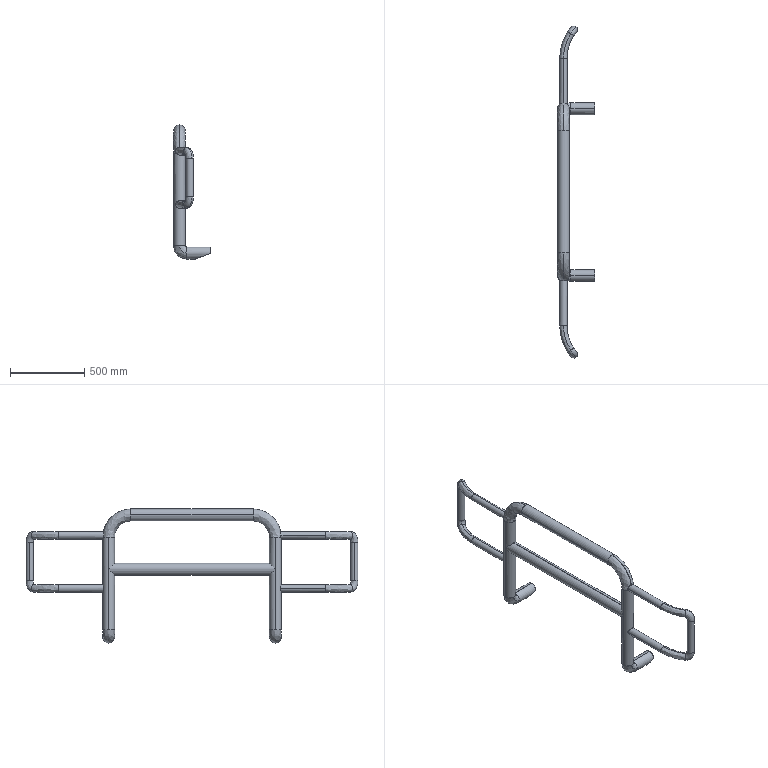Part | STEP file | Imported8 | 1 solid | 88 faces | box 248.591 x 2230 x 900 mm | volume 8406011 mm3 | cylinder 48 | spline 32 | plane 8 | commonest cylinder face diameters 50 x20 74 x14 80 x14